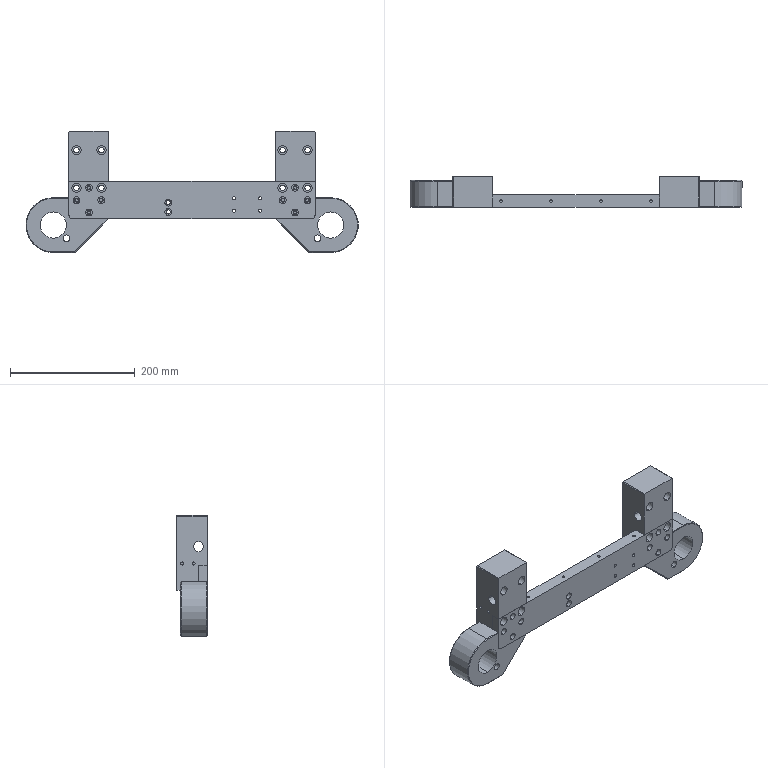Part | SolidWorks | features BaseBody 3, HoleWzd 2, ICE 2 | 3 solids | 264 faces | box 532 x 49 x 194 mm | volume 1579293 mm3 | cylinder 154 | plane 90 | cone 20 | commonest cylinder face diameters 5 x32 11 x24 15 x24 5.2 x16 6.5 x16 8.5 x16